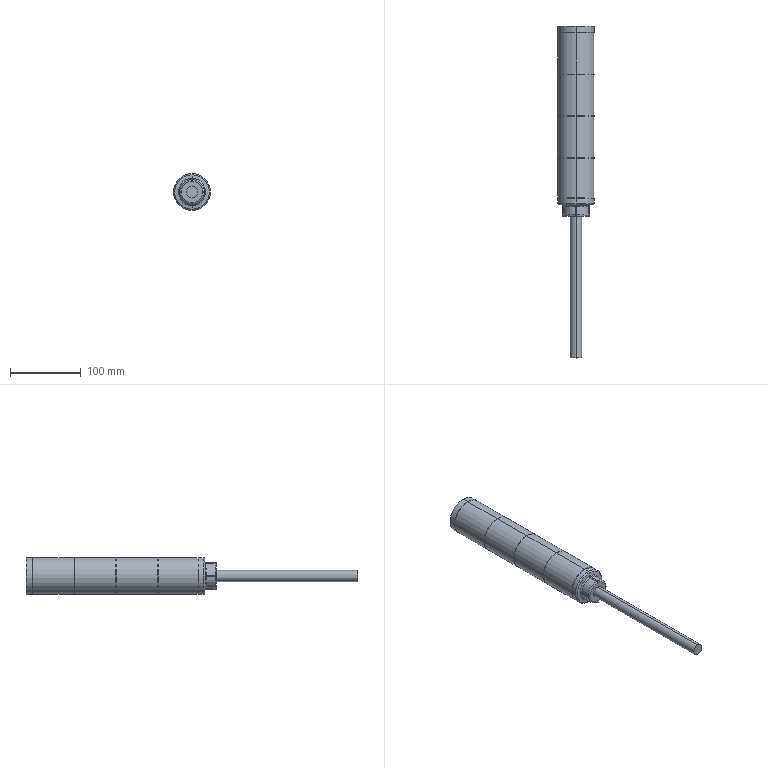Part | SolidWorks | features ICE 1, RefAxis 1, RevCut 1, Revolution 1 | 1 solid | 63 faces | box 52 x 469 x 52 mm | volume 591292 mm3 | cylinder 28 | plane 25 | torus 8 | cone 2 | commonest cylinder face diameters 52 x12 46 x10 35 x4 16 x2